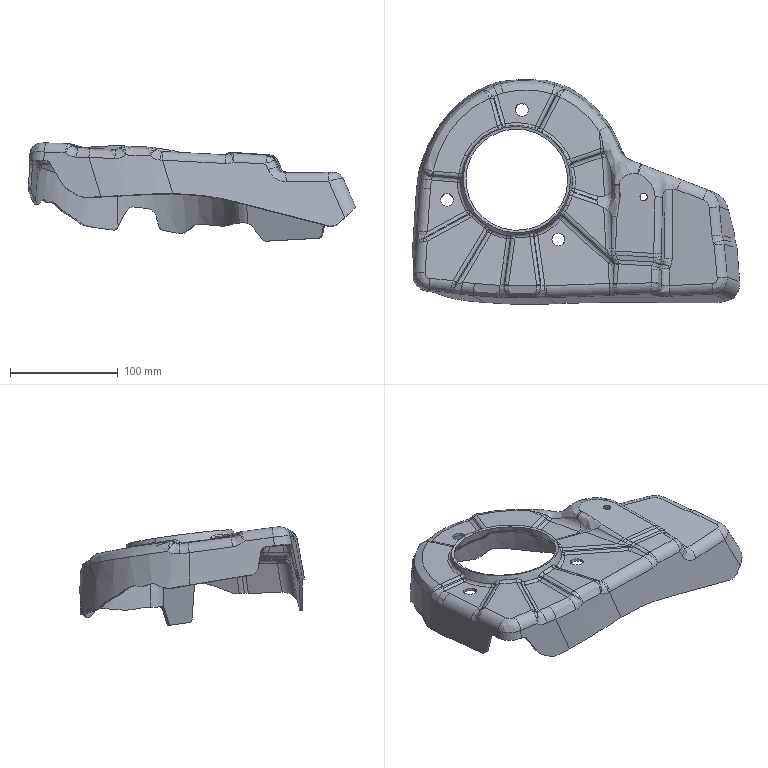Part | 1 solid | 527 faces | box 304.503 x 209.135 x 91.369 mm | volume 180005 mm3 | spline 351 | cylinder 124 | plane 47 | other 5 | commonest cylinder face diameters 15 x25 10 x20 20 x15 16 x13 5 x10 21 x9